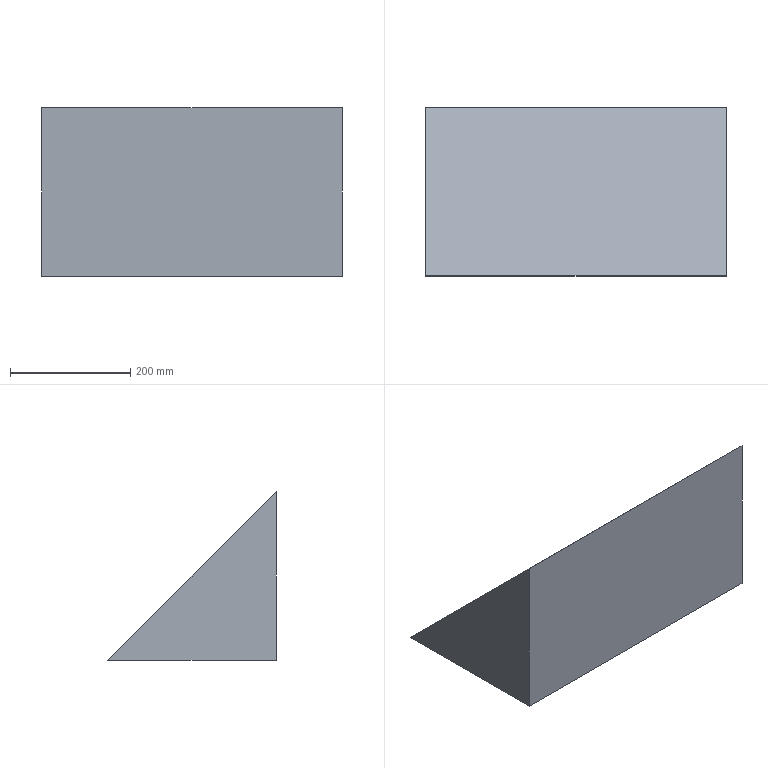Part | SolidWorks | features ICE 4, Extrusion 1 | 1 solid | 5 faces | box 500 x 280 x 280 mm | volume 19600000 mm3 | plane 5
STEP:
#1=CARTESIAN_POINT('',(460.,80.,0.));
#2=VERTEX_POINT('',#1);
#3=CARTESIAN_POINT('',(460.,-200.,0.));
#4=VERTEX_POINT('',#3);
#5=CARTESIAN_POINT('',(460.,-200.,0.));
#6=DIRECTION('',(0.,-1.,0.));
#7=VECTOR('',#6,1000.);
#8=LINE('',#5,#7);
#9=EDGE_CURVE('',#2,#4,#8,.T.);
#10=ORIENTED_EDGE('',*,*,#9,.F.);
#11=CARTESIAN_POINT('',(460.,-200.,280.));
#12=VERTEX_POINT('',#11);
#13=CARTESIAN_POINT('',(460.,-200.,280.));
#14=DIRECTION('',(0.,-0.7071,0.7071));
#15=VECTOR('',#14,1000.);
#16=LINE('',#13,#15);
#17=EDGE_CURVE('',#2,#12,#16,.T.);
#18=ORIENTED_EDGE('',*,*,#17,.T.);
#19=CARTESIAN_POINT('',(460.,-200.,0.));
#20=DIRECTION('',(0.,0.,1.));
#21=VECTOR('',#20,1000.);
#22=LINE('',#19,#21);
#23=EDGE_CURVE('',#4,#12,#22,.T.);
#24=ORIENTED_EDGE('',*,*,#23,.F.);
#25=EDGE_LOOP('',(#10,#18,#24));
#26=FACE_OUTER_BOUND('',#25,.T.);
#27=CARTESIAN_POINT('',(460.,0.,0.));
#28=DIRECTION('',(-1.,0.,0.));
#29=DIRECTION('',(0.,-1.,0.));
#30=AXIS2_PLACEMENT_3D('',#27,#28,#29);
#31=PLANE('',#30);
#32=ADVANCED_FACE('',(#26),#31,.F.);
#33=CARTESIAN_POINT('',(-40.,-200.,280.));
#34=VERTEX_POINT('',#33);
#35=CARTESIAN_POINT('',(-40.,-200.,0.));
#36=VERTEX_POINT('',#35);
#37=CARTESIAN_POINT('',(-40.,-200.,80.));
#38=DIRECTION('',(0.,0.,-1.));
#39=VECTOR('',#38,1000.);
#40=LINE('',#37,#39);
#41=EDGE_CURVE('',#34,#36,#40,.T.);
#42=ORIENTED_EDGE('',*,*,#41,.F.);
#43=CARTESIAN_POINT('',(-40.,80.,0.));
#44=VERTEX_POINT('',#43);
#45=CARTESIAN_POINT('',(-40.,100.,-20.));
#46=DIRECTION('',(0.,0.7071,-0.7071));
#47=VECTOR('',#46,1000.);
#48=LINE('',#45,#47);
#49=EDGE_CURVE('',#34,#44,#48,.T.);
#50=ORIENTED_EDGE('',*,*,#49,.T.);
#51=CARTESIAN_POINT('',(-40.,200.,0.));
#52=DIRECTION('',(0.,-1.,0.));
#53=VECTOR('',#52,1000.);
#54=LINE('',#51,#53);
#55=EDGE_CURVE('',#44,#36,#54,.T.);
#56=ORIENTED_EDGE('',*,*,#55,.T.);
#57=EDGE_LOOP('',(#42,#50,#56));
#58=FACE_OUTER_BOUND('',#57,.T.);
#59=CARTESIAN_POINT('',(-40.,200.,80.));
#60=DIRECTION('',(1.,0.,0.));
#61=DIRECTION('',(0.,1.,0.));
#62=AXIS2_PLACEMENT_3D('',#59,#60,#61);
#63=PLANE('',#62);
#64=ADVANCED_FACE('',(#58),#63,.F.);
#65=ORIENTED_EDGE('',*,*,#23,.T.);
#66=CARTESIAN_POINT('',(460.,-200.,280.));
#67=DIRECTION('',(-1.,0.,0.));
#68=VECTOR('',#67,1000.);
#69=LINE('',#66,#68);
#70=EDGE_CURVE('',#12,#34,#69,.T.);
#71=ORIENTED_EDGE('',*,*,#70,.T.);
#72=ORIENTED_EDGE('',*,*,#41,.T.);
#73=CARTESIAN_POINT('',(40.,-200.,0.));
#74=DIRECTION('',(1.,0.,0.));
#75=VECTOR('',#74,1000.);
#76=LINE('',#73,#75);
#77=EDGE_CURVE('',#36,#4,#76,.T.);
#78=ORIENTED_EDGE('',*,*,#77,.T.);
#79=EDGE_LOOP('',(#65,#71,#72,#78));
#80=FACE_OUTER_BOUND('',#79,.T.);
#81=CARTESIAN_POINT('',(40.,-200.,80.));
#82=DIRECTION('',(0.,1.,0.));
#83=DIRECTION('',(0.,0.,1.));
#84=AXIS2_PLACEMENT_3D('',#81,#82,#83);
#85=PLANE('',#84);
#86=ADVANCED_FACE('',(#80),#85,.F.);
#87=CARTESIAN_POINT('',(460.,80.,0.));
#88=DIRECTION('',(-1.,0.,0.));
#89=VECTOR('',#88,1000.);
#90=LINE('',#87,#89);
#91=EDGE_CURVE('',#2,#44,#90,.T.);
#92=ORIENTED_EDGE('',*,*,#91,.F.);
#93=ORIENTED_EDGE('',*,*,#9,.T.);
#94=ORIENTED_EDGE('',*,*,#77,.F.);
#95=ORIENTED_EDGE('',*,*,#55,.F.);
#96=EDGE_LOOP('',(#92,#93,#94,#95));
#97=FACE_OUTER_BOUND('',#96,.T.);
#98=CARTESIAN_POINT('',(0.,0.,0.));
#99=DIRECTION('',(0.,0.,-1.));
#100=DIRECTION('',(-1.,0.,0.));
#101=AXIS2_PLACEMENT_3D('',#98,#99,#100);
#102=PLANE('',#101);
#103=ADVANCED_FACE('',(#97),#102,.T.);
#104=ORIENTED_EDGE('',*,*,#70,.F.);
#105=ORIENTED_EDGE('',*,*,#17,.F.);
#106=ORIENTED_EDGE('',*,*,#91,.T.);
#107=ORIENTED_EDGE('',*,*,#49,.F.);
#108=EDGE_LOOP('',(#104,#105,#106,#107));
#109=FACE_OUTER_BOUND('',#108,.T.);
#110=CARTESIAN_POINT('',(460.,-200.,280.));
#111=DIRECTION('',(0.,-0.7071,-0.7071));
#112=DIRECTION('',(0.,0.7071,-0.7071));
#113=AXIS2_PLACEMENT_3D('',#110,#111,#112);
#114=PLANE('',#113);
#115=ADVANCED_FACE('',(#109),#114,.F.);
#116=CLOSED_SHELL('',(#32,#64,#86,#103,#115));
#117=MANIFOLD_SOLID_BREP('',#116);
#118=CARTESIAN_POINT('',(0.,0.,0.));
#119=DIRECTION('',(0.,0.,1.));
#120=DIRECTION('',(1.,0.,0.));
#121=AXIS2_PLACEMENT_3D('',#118,#119,#120);
#122=(LENGTH_UNIT()NAMED_UNIT(*)SI_UNIT(.MILLI.,.METRE.));
#123=UNCERTAINTY_MEASURE_WITH_UNIT(LENGTH_MEASURE(0.00001),#122,'','');
#124=(NAMED_UNIT(*)PLANE_ANGLE_UNIT()SI_UNIT($,.RADIAN.));
#125=(NAMED_UNIT(*)SI_UNIT($,.STERADIAN.)SOLID_ANGLE_UNIT());
#126=(GEOMETRIC_REPRESENTATION_CONTEXT(3)GLOBAL_UNCERTAINTY_ASSIGNED_CONTEXT((#123))GLOBAL_UNIT_ASSIGNED_CONTEXT((#122,#124,#125))REPRESENTATION_CONTEXT('',''));
#127=ADVANCED_BREP_SHAPE_REPRESENTATION('',(#117,#121),#126);